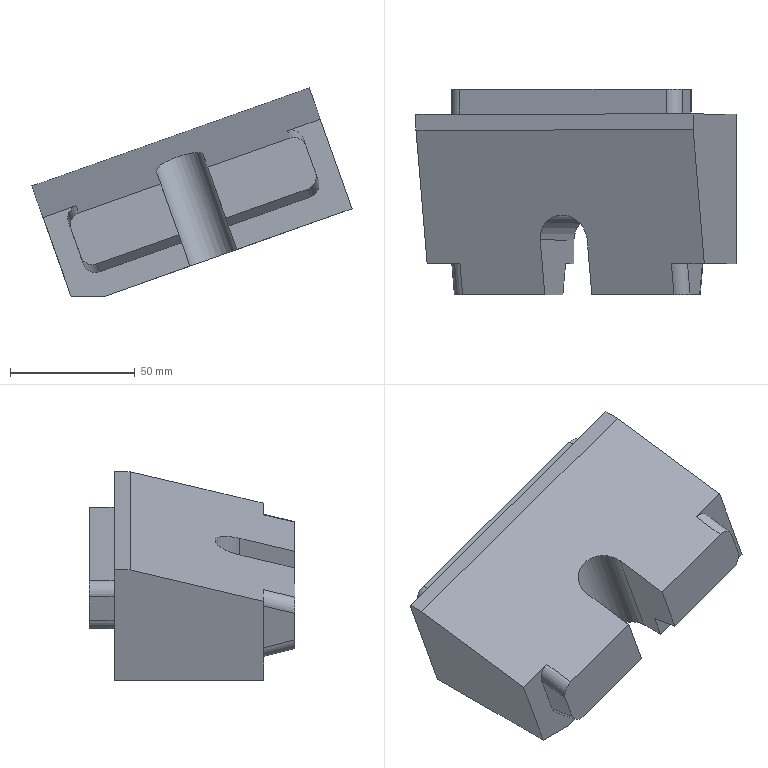Part | STEP file | WEDGE-1_id570_x_t | 1 solid | 31 faces | box 128.423 x 82.5 x 83.604 mm | volume 350596 mm3 | plane 22 | cylinder 9 | commonest cylinder face diameters 10 x8 20 x1
STEP:
#1=CARTESIAN_POINT('',(99.636,10.5,-205.83));
#2=VERTEX_POINT('',#1);
#3=CARTESIAN_POINT('',(16.683,10.5,-235.205));
#4=VERTEX_POINT('',#3);
#5=CARTESIAN_POINT('',(114.718,10.5,-200.489));
#6=DIRECTION('',(-0.9426,0.,-0.3338));
#7=VECTOR('',#6,1.);
#8=LINE('',#5,#7);
#9=EDGE_CURVE('',#2,#4,#8,.T.);
#10=ORIENTED_EDGE('',*,*,#9,.F.);
#11=CARTESIAN_POINT('',(106.018,10.5,-208.874));
#12=VERTEX_POINT('',#11);
#13=CARTESIAN_POINT('',(101.305,10.5,-210.543));
#14=DIRECTION('',(0.,-1.,0.));
#15=DIRECTION('',(0.,0.,1.));
#16=AXIS2_PLACEMENT_3D('',#13,#14,#15);
#17=CIRCLE('',#16,5.);
#18=EDGE_CURVE('',#12,#2,#17,.T.);
#19=ORIENTED_EDGE('',*,*,#18,.F.);
#20=CARTESIAN_POINT('',(109.356,10.5,-218.3));
#21=VERTEX_POINT('',#20);
#22=CARTESIAN_POINT('',(104.349,10.5,-204.16));
#23=DIRECTION('',(0.3338,0.,-0.9426));
#24=VECTOR('',#23,1.);
#25=LINE('',#22,#24);
#26=EDGE_CURVE('',#12,#21,#25,.T.);
#27=ORIENTED_EDGE('',*,*,#26,.T.);
#28=CARTESIAN_POINT('',(106.312,10.5,-224.682));
#29=VERTEX_POINT('',#28);
#30=CARTESIAN_POINT('',(104.643,10.5,-219.969));
#31=DIRECTION('',(0.,-1.,0.));
#32=DIRECTION('',(0.,0.,-1.));
#33=AXIS2_PLACEMENT_3D('',#30,#31,#32);
#34=CIRCLE('',#33,5.);
#35=EDGE_CURVE('',#29,#21,#34,.T.);
#36=ORIENTED_EDGE('',*,*,#35,.F.);
#37=CARTESIAN_POINT('',(23.359,10.5,-254.057));
#38=VERTEX_POINT('',#37);
#39=CARTESIAN_POINT('',(121.394,10.5,-219.341));
#40=DIRECTION('',(0.9426,0.,0.3338));
#41=VECTOR('',#40,1.);
#42=LINE('',#39,#41);
#43=EDGE_CURVE('',#38,#29,#42,.T.);
#44=ORIENTED_EDGE('',*,*,#43,.F.);
#45=CARTESIAN_POINT('',(16.977,10.5,-251.013));
#46=VERTEX_POINT('',#45);
#47=CARTESIAN_POINT('',(21.69,10.5,-249.344));
#48=DIRECTION('',(0.,-1.,0.));
#49=DIRECTION('',(0.,0.,1.));
#50=AXIS2_PLACEMENT_3D('',#47,#48,#49);
#51=CIRCLE('',#50,5.);
#52=EDGE_CURVE('',#46,#38,#51,.T.);
#53=ORIENTED_EDGE('',*,*,#52,.F.);
#54=CARTESIAN_POINT('',(13.639,10.5,-241.587));
#55=VERTEX_POINT('',#54);
#56=CARTESIAN_POINT('',(18.646,10.5,-255.726));
#57=DIRECTION('',(-0.3338,0.,0.9426));
#58=VECTOR('',#57,1.);
#59=LINE('',#56,#58);
#60=EDGE_CURVE('',#46,#55,#59,.T.);
#61=ORIENTED_EDGE('',*,*,#60,.T.);
#62=CARTESIAN_POINT('',(18.352,10.5,-239.918));
#63=DIRECTION('',(0.,-1.,0.));
#64=DIRECTION('',(0.,0.,-1.));
#65=AXIS2_PLACEMENT_3D('',#62,#63,#64);
#66=CIRCLE('',#65,5.);
#67=EDGE_CURVE('',#4,#55,#66,.T.);
#68=ORIENTED_EDGE('',*,*,#67,.F.);
#69=EDGE_LOOP('',(#10,#19,#27,#36,#44,#53,#61,#68));
#70=FACE_OUTER_BOUND('',#69,.T.);
#71=CARTESIAN_POINT('',(114.718,10.5,-200.489));
#72=DIRECTION('',(0.,1.,0.));
#73=DIRECTION('',(0.,0.,1.));
#74=AXIS2_PLACEMENT_3D('',#71,#72,#73);
#75=PLANE('',#74);
#76=ADVANCED_FACE('',(#70),#75,.T.);
#77=CARTESIAN_POINT('',(106.018,0.5,-208.874));
#78=VERTEX_POINT('',#77);
#79=CARTESIAN_POINT('',(99.636,0.5,-205.83));
#80=VERTEX_POINT('',#79);
#81=CARTESIAN_POINT('',(101.305,0.5,-210.543));
#82=DIRECTION('',(0.,-1.,0.));
#83=DIRECTION('',(0.,0.,1.));
#84=AXIS2_PLACEMENT_3D('',#81,#82,#83);
#85=CIRCLE('',#84,5.);
#86=EDGE_CURVE('',#78,#80,#85,.T.);
#87=ORIENTED_EDGE('',*,*,#86,.F.);
#88=CARTESIAN_POINT('',(106.018,0.5,-208.874));
#89=DIRECTION('',(0.,1.,0.));
#90=VECTOR('',#89,1.);
#91=LINE('',#88,#90);
#92=EDGE_CURVE('',#78,#12,#91,.T.);
#93=ORIENTED_EDGE('',*,*,#92,.T.);
#94=ORIENTED_EDGE('',*,*,#18,.T.);
#95=CARTESIAN_POINT('',(99.636,0.5,-205.83));
#96=DIRECTION('',(0.,1.,0.));
#97=VECTOR('',#96,1.);
#98=LINE('',#95,#97);
#99=EDGE_CURVE('',#80,#2,#98,.T.);
#100=ORIENTED_EDGE('',*,*,#99,.F.);
#101=EDGE_LOOP('',(#87,#93,#94,#100));
#102=FACE_OUTER_BOUND('',#101,.T.);
#103=CARTESIAN_POINT('',(101.305,0.2133,-210.543));
#104=DIRECTION('',(0.,1.,0.));
#105=DIRECTION('',(0.,0.,1.));
#106=AXIS2_PLACEMENT_3D('',#103,#104,#105);
#107=CYLINDRICAL_SURFACE('',#106,5.);
#108=ADVANCED_FACE('',(#102),#107,.T.);
#109=CARTESIAN_POINT('',(16.683,0.5,-235.205));
#110=VERTEX_POINT('',#109);
#111=CARTESIAN_POINT('',(99.636,0.5,-205.83));
#112=DIRECTION('',(-0.9426,0.,-0.3338));
#113=VECTOR('',#112,1.);
#114=LINE('',#111,#113);
#115=EDGE_CURVE('',#80,#110,#114,.T.);
#116=ORIENTED_EDGE('',*,*,#115,.F.);
#117=ORIENTED_EDGE('',*,*,#99,.T.);
#118=ORIENTED_EDGE('',*,*,#9,.T.);
#119=CARTESIAN_POINT('',(16.683,10.738,-235.205));
#120=DIRECTION('',(0.,1.,0.));
#121=VECTOR('',#120,1.);
#122=LINE('',#119,#121);
#123=EDGE_CURVE('',#110,#4,#122,.T.);
#124=ORIENTED_EDGE('',*,*,#123,.F.);
#125=EDGE_LOOP('',(#116,#117,#118,#124));
#126=FACE_OUTER_BOUND('',#125,.T.);
#127=CARTESIAN_POINT('',(114.718,0.5,-200.489));
#128=DIRECTION('',(-0.3338,0.,0.9426));
#129=DIRECTION('',(0.9426,0.,0.3338));
#130=AXIS2_PLACEMENT_3D('',#127,#128,#129);
#131=PLANE('',#130);
#132=ADVANCED_FACE('',(#126),#131,.T.);
#133=ORIENTED_EDGE('',*,*,#67,.T.);
#134=CARTESIAN_POINT('',(13.639,0.5,-241.587));
#135=VERTEX_POINT('',#134);
#136=CARTESIAN_POINT('',(13.639,0.5,-241.587));
#137=DIRECTION('',(0.,-1.,0.));
#138=VECTOR('',#137,1.);
#139=LINE('',#136,#138);
#140=EDGE_CURVE('',#55,#135,#139,.T.);
#141=ORIENTED_EDGE('',*,*,#140,.T.);
#142=CARTESIAN_POINT('',(18.352,0.5,-239.918));
#143=DIRECTION('',(0.,-1.,0.));
#144=DIRECTION('',(0.,0.,-1.));
#145=AXIS2_PLACEMENT_3D('',#142,#143,#144);
#146=CIRCLE('',#145,5.);
#147=EDGE_CURVE('',#110,#135,#146,.T.);
#148=ORIENTED_EDGE('',*,*,#147,.F.);
#149=ORIENTED_EDGE('',*,*,#123,.T.);
#150=EDGE_LOOP('',(#133,#141,#148,#149));
#151=FACE_OUTER_BOUND('',#150,.T.);
#152=CARTESIAN_POINT('',(18.352,10.738,-239.918));
#153=DIRECTION('',(0.,-1.,0.));
#154=DIRECTION('',(0.,0.,-1.));
#155=AXIS2_PLACEMENT_3D('',#152,#153,#154);
#156=CYLINDRICAL_SURFACE('',#155,5.);
#157=ADVANCED_FACE('',(#151),#156,.T.);
#158=CARTESIAN_POINT('',(16.977,0.5,-251.013));
#159=VERTEX_POINT('',#158);
#160=CARTESIAN_POINT('',(16.977,0.237,-251.013));
#161=DIRECTION('',(0.,1.,0.));
#162=VECTOR('',#161,1.);
#163=LINE('',#160,#162);
#164=EDGE_CURVE('',#159,#46,#163,.T.);
#165=ORIENTED_EDGE('',*,*,#164,.F.);
#166=CARTESIAN_POINT('',(13.639,0.5,-241.587));
#167=DIRECTION('',(0.3338,0.,-0.9426));
#168=VECTOR('',#167,1.);
#169=LINE('',#166,#168);
#170=EDGE_CURVE('',#135,#159,#169,.T.);
#171=ORIENTED_EDGE('',*,*,#170,.F.);
#172=ORIENTED_EDGE('',*,*,#140,.F.);
#173=ORIENTED_EDGE('',*,*,#60,.F.);
#174=EDGE_LOOP('',(#165,#171,#172,#173));
#175=FACE_OUTER_BOUND('',#174,.T.);
#176=CARTESIAN_POINT('',(18.646,0.5,-255.726));
#177=DIRECTION('',(0.9426,0.,0.3338));
#178=DIRECTION('',(0.3338,0.,-0.9426));
#179=AXIS2_PLACEMENT_3D('',#176,#177,#178);
#180=PLANE('',#179);
#181=ADVANCED_FACE('',(#175),#180,.F.);
#182=CARTESIAN_POINT('',(23.359,0.5,-254.057));
#183=VERTEX_POINT('',#182);
#184=CARTESIAN_POINT('',(21.69,0.5,-249.344));
#185=DIRECTION('',(0.,-1.,0.));
#186=DIRECTION('',(0.,0.,1.));
#187=AXIS2_PLACEMENT_3D('',#184,#185,#186);
#188=CIRCLE('',#187,5.);
#189=EDGE_CURVE('',#159,#183,#188,.T.);
#190=ORIENTED_EDGE('',*,*,#189,.F.);
#191=ORIENTED_EDGE('',*,*,#164,.T.);
#192=ORIENTED_EDGE('',*,*,#52,.T.);
#193=CARTESIAN_POINT('',(23.359,10.5,-254.057));
#194=DIRECTION('',(0.,1.,0.));
#195=VECTOR('',#194,1.);
#196=LINE('',#193,#195);
#197=EDGE_CURVE('',#183,#38,#196,.T.);
#198=ORIENTED_EDGE('',*,*,#197,.F.);
#199=EDGE_LOOP('',(#190,#191,#192,#198));
#200=FACE_OUTER_BOUND('',#199,.T.);
#201=CARTESIAN_POINT('',(21.69,0.237,-249.344));
#202=DIRECTION('',(0.,1.,0.));
#203=DIRECTION('',(0.,0.,1.));
#204=AXIS2_PLACEMENT_3D('',#201,#202,#203);
#205=CYLINDRICAL_SURFACE('',#204,5.);
#206=ADVANCED_FACE('',(#200),#205,.T.);
#207=ORIENTED_EDGE('',*,*,#43,.T.);
#208=CARTESIAN_POINT('',(106.312,0.5,-224.682));
#209=VERTEX_POINT('',#208);
#210=CARTESIAN_POINT('',(106.312,10.738,-224.682));
#211=DIRECTION('',(0.,1.,0.));
#212=VECTOR('',#211,1.);
#213=LINE('',#210,#212);
#214=EDGE_CURVE('',#209,#29,#213,.T.);
#215=ORIENTED_EDGE('',*,*,#214,.F.);
#216=CARTESIAN_POINT('',(23.359,0.5,-254.057));
#217=DIRECTION('',(0.9426,0.,0.3338));
#218=VECTOR('',#217,1.);
#219=LINE('',#216,#218);
#220=EDGE_CURVE('',#183,#209,#219,.T.);
#221=ORIENTED_EDGE('',*,*,#220,.F.);
#222=ORIENTED_EDGE('',*,*,#197,.T.);
#223=EDGE_LOOP('',(#207,#215,#221,#222));
#224=FACE_OUTER_BOUND('',#223,.T.);
#225=CARTESIAN_POINT('',(121.394,10.5,-219.341));
#226=DIRECTION('',(0.3338,0.,-0.9426));
#227=DIRECTION('',(-0.9426,0.,-0.3338));
#228=AXIS2_PLACEMENT_3D('',#225,#226,#227);
#229=PLANE('',#228);
#230=ADVANCED_FACE('',(#224),#229,.T.);
#231=ORIENTED_EDGE('',*,*,#35,.T.);
#232=CARTESIAN_POINT('',(109.356,0.5,-218.3));
#233=VERTEX_POINT('',#232);
#234=CARTESIAN_POINT('',(109.356,0.5,-218.3));
#235=DIRECTION('',(0.,-1.,0.));
#236=VECTOR('',#235,1.);
#237=LINE('',#234,#236);
#238=EDGE_CURVE('',#21,#233,#237,.T.);
#239=ORIENTED_EDGE('',*,*,#238,.T.);
#240=CARTESIAN_POINT('',(104.643,0.5,-219.969));
#241=DIRECTION('',(0.,-1.,0.));
#242=DIRECTION('',(0.,0.,-1.));
#243=AXIS2_PLACEMENT_3D('',#240,#241,#242);
#244=CIRCLE('',#243,5.);
#245=EDGE_CURVE('',#209,#233,#244,.T.);
#246=ORIENTED_EDGE('',*,*,#245,.F.);
#247=ORIENTED_EDGE('',*,*,#214,.T.);
#248=EDGE_LOOP('',(#231,#239,#246,#247));
#249=FACE_OUTER_BOUND('',#248,.T.);
#250=CARTESIAN_POINT('',(104.643,10.738,-219.969));
#251=DIRECTION('',(0.,-1.,0.));
#252=DIRECTION('',(0.,0.,-1.));
#253=AXIS2_PLACEMENT_3D('',#250,#251,#252);
#254=CYLINDRICAL_SURFACE('',#253,5.);
#255=ADVANCED_FACE('',(#249),#254,.T.);
#256=ORIENTED_EDGE('',*,*,#238,.F.);
#257=ORIENTED_EDGE('',*,*,#26,.F.);
#258=ORIENTED_EDGE('',*,*,#92,.F.);
#259=CARTESIAN_POINT('',(109.356,0.5,-218.3));
#260=DIRECTION('',(-0.3338,0.,0.9426));
#261=VECTOR('',#260,1.);
#262=LINE('',#259,#261);
#263=EDGE_CURVE('',#233,#78,#262,.T.);
#264=ORIENTED_EDGE('',*,*,#263,.F.);
#265=EDGE_LOOP('',(#256,#257,#258,#264));
#266=FACE_OUTER_BOUND('',#265,.T.);
#267=CARTESIAN_POINT('',(104.349,0.5,-204.16));
#268=DIRECTION('',(-0.9426,0.,-0.3338));
#269=DIRECTION('',(-0.3338,0.,0.9426));
#270=AXIS2_PLACEMENT_3D('',#267,#268,#269);
#271=PLANE('',#270);
#272=ADVANCED_FACE('',(#266),#271,.F.);
#273=CARTESIAN_POINT('',(109.174,-72.,-214.791));
#274=VERTEX_POINT('',#273);
#275=CARTESIAN_POINT('',(108.134,-59.5,-211.853));
#276=VERTEX_POINT('',#275);
#277=CARTESIAN_POINT('',(109.215,-72.495,-214.907));
#278=DIRECTION('',(-0.08076,0.9703,0.228));
#279=VECTOR('',#278,1.);
#280=LINE('',#277,#279);
#281=EDGE_CURVE('',#274,#276,#280,.T.);
#282=ORIENTED_EDGE('',*,*,#281,.F.);
#283=CARTESIAN_POINT('',(112.96,-72.,-225.483));
#284=VERTEX_POINT('',#283);
#285=CARTESIAN_POINT('',(112.96,-72.,-225.483));
#286=DIRECTION('',(-0.3338,0.,0.9426));
#287=VECTOR('',#286,1.);
#288=LINE('',#285,#287);
#289=EDGE_CURVE('',#284,#274,#288,.T.);
#290=ORIENTED_EDGE('',*,*,#289,.F.);
#291=CARTESIAN_POINT('',(114.078,-59.5,-228.64));
#292=VERTEX_POINT('',#291);
#293=CARTESIAN_POINT('',(114.222,-57.895,-229.046));
#294=DIRECTION('',(-0.0864,-0.9659,0.244));
#295=VECTOR('',#294,1.);
#296=LINE('',#293,#295);
#297=EDGE_CURVE('',#292,#284,#296,.T.);
#298=ORIENTED_EDGE('',*,*,#297,.F.);
#299=CARTESIAN_POINT('',(108.134,-59.5,-211.853));
#300=DIRECTION('',(0.3338,0.,-0.9426));
#301=VECTOR('',#300,1.);
#302=LINE('',#299,#301);
#303=EDGE_CURVE('',#276,#292,#302,.T.);
#304=ORIENTED_EDGE('',*,*,#303,.F.);
#305=EDGE_LOOP('',(#282,#290,#298,#304));
#306=FACE_OUTER_BOUND('',#305,.T.);
#307=CARTESIAN_POINT('',(104.791,-72.,-202.413));
#308=DIRECTION('',(-0.9426,0.,-0.3338));
#309=DIRECTION('',(-0.3338,0.,0.9426));
#310=AXIS2_PLACEMENT_3D('',#307,#308,#309);
#311=PLANE('',#310);
#312=ADVANCED_FACE('',(#306),#311,.F.);
#313=CARTESIAN_POINT('',(111.093,-59.5,-235.189));
#314=VERTEX_POINT('',#313);
#315=CARTESIAN_POINT('',(109.365,-59.5,-230.309));
#316=DIRECTION('',(0.,1.,0.));
#317=DIRECTION('',(-0.3338,0.,0.9426));
#318=AXIS2_PLACEMENT_3D('',#315,#316,#317);
#319=ELLIPSE('',#318,5.176,5.);
#320=EDGE_CURVE('',#292,#314,#319,.T.);
#321=ORIENTED_EDGE('',*,*,#320,.F.);
#322=ORIENTED_EDGE('',*,*,#297,.T.);
#323=CARTESIAN_POINT('',(109.975,-72.,-232.032));
#324=VERTEX_POINT('',#323);
#325=CARTESIAN_POINT('',(108.247,-72.,-227.152));
#326=DIRECTION('',(0.,-1.,0.));
#327=DIRECTION('',(-0.3338,0.,0.9426));
#328=AXIS2_PLACEMENT_3D('',#325,#326,#327);
#329=ELLIPSE('',#328,5.176,5.);
#330=EDGE_CURVE('',#324,#284,#329,.T.);
#331=ORIENTED_EDGE('',*,*,#330,.F.);
#332=CARTESIAN_POINT('',(111.093,-59.5,-235.189));
#333=DIRECTION('',(-0.0864,-0.9659,0.244));
#334=VECTOR('',#333,1.);
#335=LINE('',#332,#334);
#336=EDGE_CURVE('',#314,#324,#335,.T.);
#337=ORIENTED_EDGE('',*,*,#336,.F.);
#338=EDGE_LOOP('',(#321,#322,#331,#337));
#339=FACE_OUTER_BOUND('',#338,.T.);
#340=CARTESIAN_POINT('',(109.509,-57.895,-230.715));
#341=DIRECTION('',(-0.0864,-0.9659,0.244));
#342=DIRECTION('',(0.,-0.2449,-0.9696));
#343=AXIS2_PLACEMENT_3D('',#340,#341,#342);
#344=CYLINDRICAL_SURFACE('',#343,5.);
#345=ADVANCED_FACE('',(#339),#344,.T.);
#346=CARTESIAN_POINT('',(76.983,-72.,-243.715));
#347=VERTEX_POINT('',#346);
#348=CARTESIAN_POINT('',(76.983,-72.,-243.715));
#349=DIRECTION('',(0.9426,0.,0.3338));
#350=VECTOR('',#349,1.);
#351=LINE('',#348,#350);
#352=EDGE_CURVE('',#347,#324,#351,.T.);
#353=ORIENTED_EDGE('',*,*,#352,.F.);
#354=CARTESIAN_POINT('',(78.101,-59.5,-246.872));
#355=VERTEX_POINT('',#354);
#356=CARTESIAN_POINT('',(76.983,-72.,-243.715));
#357=DIRECTION('',(0.0864,0.9659,-0.244));
#358=VECTOR('',#357,1.);
#359=LINE('',#356,#358);
#360=EDGE_CURVE('',#347,#355,#359,.T.);
#361=ORIENTED_EDGE('',*,*,#360,.T.);
#362=CARTESIAN_POINT('',(111.093,-59.5,-235.189));
#363=DIRECTION('',(-0.9426,0.,-0.3338));
#364=VECTOR('',#363,1.);
#365=LINE('',#362,#364);
#366=EDGE_CURVE('',#314,#355,#365,.T.);
#367=ORIENTED_EDGE('',*,*,#366,.F.);
#368=ORIENTED_EDGE('',*,*,#336,.T.);
#369=EDGE_LOOP('',(#353,#361,#367,#368));
#370=FACE_OUTER_BOUND('',#369,.T.);
#371=CARTESIAN_POINT('',(125.233,-59.5,-230.182));
#372=DIRECTION('',(0.3224,-0.2588,-0.9105));
#373=DIRECTION('',(-0.9426,0.,-0.3338));
#374=AXIS2_PLACEMENT_3D('',#371,#372,#373);
#375=PLANE('',#374);
#376=ADVANCED_FACE('',(#370),#375,.T.);
#377=ORIENTED_EDGE('',*,*,#245,.T.);
#378=ORIENTED_EDGE('',*,*,#263,.T.);
#379=ORIENTED_EDGE('',*,*,#86,.T.);
#380=ORIENTED_EDGE('',*,*,#115,.T.);
#381=ORIENTED_EDGE('',*,*,#147,.T.);
#382=ORIENTED_EDGE('',*,*,#170,.T.);
#383=ORIENTED_EDGE('',*,*,#189,.T.);
#384=ORIENTED_EDGE('',*,*,#220,.T.);
#385=EDGE_LOOP('',(#377,#378,#379,#380,#381,#382,#383,#384));
#386=FACE_BOUND('',#385,.T.);
#387=CARTESIAN_POINT('',(28.628,0.5,-275.));
#388=VERTEX_POINT('',#387);
#389=CARTESIAN_POINT('',(14.863,0.5,-275.));
#390=VERTEX_POINT('',#389);
#391=CARTESIAN_POINT('',(14.863,0.5,-275.));
#392=DIRECTION('',(-1.,0.,0.));
#393=VECTOR('',#392,1.);
#394=LINE('',#391,#393);
#395=EDGE_CURVE('',#388,#390,#394,.T.);
#396=ORIENTED_EDGE('',*,*,#395,.T.);
#397=CARTESIAN_POINT('',(-0.7945,0.5,-230.785));
#398=VERTEX_POINT('',#397);
#399=CARTESIAN_POINT('',(16.397,0.5,-279.331));
#400=DIRECTION('',(-0.3338,0.,0.9426));
#401=VECTOR('',#400,1.);
#402=LINE('',#399,#401);
#403=EDGE_CURVE('',#390,#398,#402,.T.);
#404=ORIENTED_EDGE('',*,*,#403,.T.);
#405=CARTESIAN_POINT('',(110.437,0.5,-191.396));
#406=VERTEX_POINT('',#405);
#407=CARTESIAN_POINT('',(111.38,0.5,-191.062));
#408=DIRECTION('',(-0.9426,0.,-0.3338));
#409=VECTOR('',#408,1.);
#410=LINE('',#407,#409);
#411=EDGE_CURVE('',#406,#398,#410,.T.);
#412=ORIENTED_EDGE('',*,*,#411,.F.);
#413=CARTESIAN_POINT('',(127.628,0.5,-239.942));
#414=VERTEX_POINT('',#413);
#415=CARTESIAN_POINT('',(127.628,0.5,-239.942));
#416=DIRECTION('',(0.3338,0.,-0.9426));
#417=VECTOR('',#416,1.);
#418=LINE('',#415,#417);
#419=EDGE_CURVE('',#406,#414,#418,.T.);
#420=ORIENTED_EDGE('',*,*,#419,.T.);
#421=CARTESIAN_POINT('',(128.571,0.5,-239.608));
#422=DIRECTION('',(0.9426,0.,0.3338));
#423=VECTOR('',#422,1.);
#424=LINE('',#421,#423);
#425=EDGE_CURVE('',#388,#414,#424,.T.);
#426=ORIENTED_EDGE('',*,*,#425,.F.);
#427=EDGE_LOOP('',(#396,#404,#412,#420,#426));
#428=FACE_BOUND('',#427,.T.);
#429=CARTESIAN_POINT('',(111.38,0.5,-191.062));
#430=DIRECTION('',(0.,1.,0.));
#431=DIRECTION('',(0.,0.,1.));
#432=AXIS2_PLACEMENT_3D('',#429,#430,#431);
#433=PLANE('',#432);
#434=ADVANCED_FACE('',(#386,#428),#433,.T.);
#435=ORIENTED_EDGE('',*,*,#395,.F.);
#436=CARTESIAN_POINT('',(28.628,-59.5,-275.));
#437=VERTEX_POINT('',#436);
#438=CARTESIAN_POINT('',(28.628,0.5,-275.));
#439=DIRECTION('',(0.,1.,0.));
#440=VECTOR('',#439,1.);
#441=LINE('',#438,#440);
#442=EDGE_CURVE('',#437,#388,#441,.T.);
#443=ORIENTED_EDGE('',*,*,#442,.F.);
#444=CARTESIAN_POINT('',(14.863,-59.5,-275.));
#445=VERTEX_POINT('',#444);
#446=CARTESIAN_POINT('',(128.571,-59.5,-275.));
#447=DIRECTION('',(1.,0.,0.));
#448=VECTOR('',#447,1.);
#449=LINE('',#446,#448);
#450=EDGE_CURVE('',#445,#437,#449,.T.);
#451=ORIENTED_EDGE('',*,*,#450,.F.);
#452=CARTESIAN_POINT('',(14.863,10.5,-275.));
#453=DIRECTION('',(0.,1.,0.));
#454=VECTOR('',#453,1.);
#455=LINE('',#452,#454);
#456=EDGE_CURVE('',#445,#390,#455,.T.);
#457=ORIENTED_EDGE('',*,*,#456,.T.);
#458=EDGE_LOOP('',(#435,#443,#451,#457));
#459=FACE_OUTER_BOUND('',#458,.T.);
#460=CARTESIAN_POINT('',(14.863,0.5,-275.));
#461=DIRECTION('',(0.,0.,1.));
#462=DIRECTION('',(1.,0.,0.));
#463=AXIS2_PLACEMENT_3D('',#460,#461,#462);
#464=PLANE('',#463);
#465=ADVANCED_FACE('',(#459),#464,.F.);
#466=CARTESIAN_POINT('',(18.696,-72.,-258.864));
#467=VERTEX_POINT('',#466);
#468=CARTESIAN_POINT('',(19.814,-59.5,-262.021));
#469=VERTEX_POINT('',#468);
#470=CARTESIAN_POINT('',(18.657,-72.437,-258.753));
#471=DIRECTION('',(0.0864,0.9659,-0.244));
#472=VECTOR('',#471,1.);
#473=LINE('',#470,#472);
#474=EDGE_CURVE('',#467,#469,#473,.T.);
#475=ORIENTED_EDGE('',*,*,#474,.F.);
#476=CARTESIAN_POINT('',(14.91,-72.,-248.172));
#477=VERTEX_POINT('',#476);
#478=CARTESIAN_POINT('',(14.91,-72.,-248.172));
#479=DIRECTION('',(0.3338,0.,-0.9426));
#480=VECTOR('',#479,1.);
#481=LINE('',#478,#480);
#482=EDGE_CURVE('',#477,#467,#481,.T.);
#483=ORIENTED_EDGE('',*,*,#482,.F.);
#484=CARTESIAN_POINT('',(13.87,-59.5,-245.234));
#485=VERTEX_POINT('',#484);
#486=CARTESIAN_POINT('',(9.275,-4.289,-232.258));
#487=DIRECTION('',(0.08076,-0.9703,-0.228));
#488=VECTOR('',#487,1.);
#489=LINE('',#486,#488);
#490=EDGE_CURVE('',#485,#477,#489,.T.);
#491=ORIENTED_EDGE('',*,*,#490,.F.);
#492=CARTESIAN_POINT('',(19.814,-59.5,-262.021));
#493=DIRECTION('',(-0.3338,0.,0.9426));
#494=VECTOR('',#493,1.);
#495=LINE('',#492,#494);
#496=EDGE_CURVE('',#469,#485,#495,.T.);
#497=ORIENTED_EDGE('',*,*,#496,.F.);
#498=EDGE_LOOP('',(#475,#483,#491,#497));
#499=FACE_OUTER_BOUND('',#498,.T.);
#500=CARTESIAN_POINT('',(24.88,-72.,-276.327));
#501=DIRECTION('',(0.9426,0.,0.3338));
#502=DIRECTION('',(0.3338,0.,-0.9426));
#503=AXIS2_PLACEMENT_3D('',#500,#501,#502);
#504=PLANE('',#503);
#505=ADVANCED_FACE('',(#499),#504,.F.);
#506=CARTESIAN_POINT('',(25.137,-72.,-262.074));
#507=VERTEX_POINT('',#506);
#508=CARTESIAN_POINT('',(23.409,-72.,-257.195));
#509=DIRECTION('',(0.,-1.,0.));
#510=DIRECTION('',(0.3338,0.,-0.9426));
#511=AXIS2_PLACEMENT_3D('',#508,#509,#510);
#512=ELLIPSE('',#511,5.176,5.);
#513=EDGE_CURVE('',#467,#507,#512,.T.);
#514=ORIENTED_EDGE('',*,*,#513,.F.);
#515=ORIENTED_EDGE('',*,*,#474,.T.);
#516=CARTESIAN_POINT('',(26.255,-59.5,-265.232));
#517=VERTEX_POINT('',#516);
#518=CARTESIAN_POINT('',(24.528,-59.5,-260.352));
#519=DIRECTION('',(0.,1.,0.));
#520=DIRECTION('',(0.3338,0.,-0.9426));
#521=AXIS2_PLACEMENT_3D('',#518,#519,#520);
#522=ELLIPSE('',#521,5.176,5.);
#523=EDGE_CURVE('',#517,#469,#522,.T.);
#524=ORIENTED_EDGE('',*,*,#523,.F.);
#525=CARTESIAN_POINT('',(26.255,-59.5,-265.232));
#526=DIRECTION('',(0.0864,0.9659,-0.244));
#527=VECTOR('',#526,1.);
#528=LINE('',#525,#527);
#529=EDGE_CURVE('',#507,#517,#528,.T.);
#530=ORIENTED_EDGE('',*,*,#529,.F.);
#531=EDGE_LOOP('',(#514,#515,#524,#530));
#532=FACE_OUTER_BOUND('',#531,.T.);
#533=CARTESIAN_POINT('',(23.37,-72.437,-257.084));
#534=DIRECTION('',(0.0864,0.9659,-0.244));
#535=DIRECTION('',(0.,0.2449,0.9696));
#536=AXIS2_PLACEMENT_3D('',#533,#534,#535);
#537=CYLINDRICAL_SURFACE('',#536,5.);
#538=ADVANCED_FACE('',(#532),#537,.T.);
#539=CARTESIAN_POINT('',(59.248,-59.5,-253.548));
#540=VERTEX_POINT('',#539);
#541=CARTESIAN_POINT('',(59.248,-59.5,-253.548));
#542=DIRECTION('',(-0.9426,0.,-0.3338));
#543=VECTOR('',#542,1.);
#544=LINE('',#541,#543);
#545=EDGE_CURVE('',#540,#517,#544,.T.);
#546=ORIENTED_EDGE('',*,*,#545,.F.);
#547=CARTESIAN_POINT('',(58.13,-72.,-250.391));
#548=VERTEX_POINT('',#547);
#549=CARTESIAN_POINT('',(59.248,-59.5,-253.548));
#550=DIRECTION('',(-0.0864,-0.9659,0.244));
#551=VECTOR('',#550,1.);
#552=LINE('',#549,#551);
#553=EDGE_CURVE('',#540,#548,#552,.T.);
#554=ORIENTED_EDGE('',*,*,#553,.T.);
#555=CARTESIAN_POINT('',(25.137,-72.,-262.074));
#556=DIRECTION('',(0.9426,0.,0.3338));
#557=VECTOR('',#556,1.);
#558=LINE('',#555,#557);
#559=EDGE_CURVE('',#507,#548,#558,.T.);
#560=ORIENTED_EDGE('',*,*,#559,.F.);
#561=ORIENTED_EDGE('',*,*,#529,.T.);
#562=EDGE_LOOP('',(#546,#554,#560,#561));
#563=FACE_OUTER_BOUND('',#562,.T.);
#564=CARTESIAN_POINT('',(125.233,-59.5,-230.182));
#565=DIRECTION('',(0.3224,-0.2588,-0.9105));
#566=DIRECTION('',(-0.9426,0.,-0.3338));
#567=AXIS2_PLACEMENT_3D('',#564,#565,#566);
#568=PLANE('',#567);
#569=ADVANCED_FACE('',(#563),#568,.T.);
#570=CARTESIAN_POINT('',(81.439,-59.5,-256.299));
#571=VERTEX_POINT('',#570);
#572=CARTESIAN_POINT('',(81.439,-50.,-256.299));
#573=VERTEX_POINT('',#572);
#574=CARTESIAN_POINT('',(81.439,-76.822,-256.299));
#575=DIRECTION('',(0.,1.,0.));
#576=VECTOR('',#575,1.);
#577=LINE('',#574,#576);
#578=EDGE_CURVE('',#571,#573,#577,.T.);
#579=ORIENTED_EDGE('',*,*,#578,.T.);
#580=CARTESIAN_POINT('',(62.586,-50.,-262.975));
#581=VERTEX_POINT('',#580);
#582=CARTESIAN_POINT('',(72.012,-50.,-259.637));
#583=DIRECTION('',(-0.3338,0.,0.9426));
#584=DIRECTION('',(0.9426,0.,0.3338));
#585=AXIS2_PLACEMENT_3D('',#582,#583,#584);
#586=CIRCLE('',#585,10.);
#587=EDGE_CURVE('',#573,#581,#586,.T.);
#588=ORIENTED_EDGE('',*,*,#587,.T.);
#589=CARTESIAN_POINT('',(62.586,-59.5,-262.975));
#590=VERTEX_POINT('',#589);
#591=CARTESIAN_POINT('',(62.586,-50.,-262.975));
#592=DIRECTION('',(0.,-1.,0.));
#593=VECTOR('',#592,1.);
#594=LINE('',#591,#593);
#595=EDGE_CURVE('',#581,#590,#594,.T.);
#596=ORIENTED_EDGE('',*,*,#595,.T.);
#597=CARTESIAN_POINT('',(28.628,-59.5,-275.));
#598=DIRECTION('',(0.9426,0.,0.3338));
#599=VECTOR('',#598,1.);
#600=LINE('',#597,#599);
#601=EDGE_CURVE('',#437,#590,#600,.T.);
#602=ORIENTED_EDGE('',*,*,#601,.F.);
#603=ORIENTED_EDGE('',*,*,#442,.T.);
#604=ORIENTED_EDGE('',*,*,#425,.T.);
#605=CARTESIAN_POINT('',(127.628,-59.5,-239.942));
#606=VERTEX_POINT('',#605);
#607=CARTESIAN_POINT('',(127.628,-72.,-239.942));
#608=DIRECTION('',(0.,-1.,0.));
#609=VECTOR('',#608,1.);
#610=LINE('',#607,#609);
#611=EDGE_CURVE('',#414,#606,#610,.T.);
#612=ORIENTED_EDGE('',*,*,#611,.T.);
#613=CARTESIAN_POINT('',(81.439,-59.5,-256.299));
#614=DIRECTION('',(0.9426,0.,0.3338));
#615=VECTOR('',#614,1.);
#616=LINE('',#613,#615);
#617=EDGE_CURVE('',#571,#606,#616,.T.);
#618=ORIENTED_EDGE('',*,*,#617,.F.);
#619=EDGE_LOOP('',(#579,#588,#596,#602,#603,#604,#612,#618));
#620=FACE_OUTER_BOUND('',#619,.T.);
#621=CARTESIAN_POINT('',(128.571,0.5,-239.608));
#622=DIRECTION('',(0.3338,0.,-0.9426));
#623=DIRECTION('',(-0.9426,0.,-0.3338));
#624=AXIS2_PLACEMENT_3D('',#621,#622,#623);
#625=PLANE('',#624);
#626=ADVANCED_FACE('',(#620),#625,.T.);
#627=ORIENTED_EDGE('',*,*,#578,.F.);
#628=CARTESIAN_POINT('',(78.101,-59.5,-246.872));
#629=DIRECTION('',(0.3338,0.,-0.9426));
#630=VECTOR('',#629,1.);
#631=LINE('',#628,#630);
#632=EDGE_CURVE('',#355,#571,#631,.T.);
#633=ORIENTED_EDGE('',*,*,#632,.F.);
#634=ORIENTED_EDGE('',*,*,#360,.F.);
#635=CARTESIAN_POINT('',(69.748,-72.,-223.286));
#636=VERTEX_POINT('',#635);
#637=CARTESIAN_POINT('',(69.748,-72.,-223.286));
#638=DIRECTION('',(0.3338,0.,-0.9426));
#639=VECTOR('',#638,1.);
#640=LINE('',#637,#639);
#641=EDGE_CURVE('',#636,#347,#640,.T.);
#642=ORIENTED_EDGE('',*,*,#641,.F.);
#643=CARTESIAN_POINT('',(67.917,-50.,-218.115));
#644=VERTEX_POINT('',#643);
#645=CARTESIAN_POINT('',(69.748,-72.,-223.286));
#646=DIRECTION('',(0.08076,-0.9703,-0.228));
#647=VECTOR('',#646,1.);
#648=LINE('',#645,#647);
#649=EDGE_CURVE('',#644,#636,#648,.T.);
#650=ORIENTED_EDGE('',*,*,#649,.F.);
#651=CARTESIAN_POINT('',(64.248,-50.,-207.753));
#652=DIRECTION('',(0.3338,0.,-0.9426));
#653=VECTOR('',#652,1.);
#654=LINE('',#651,#653);
#655=EDGE_CURVE('',#644,#573,#654,.T.);
#656=ORIENTED_EDGE('',*,*,#655,.T.);
#657=EDGE_LOOP('',(#627,#633,#634,#642,#650,#656));
#658=FACE_OUTER_BOUND('',#657,.T.);
#659=CARTESIAN_POINT('',(64.248,-76.822,-207.753));
#660=DIRECTION('',(0.9426,0.,0.3338));
#661=DIRECTION('',(0.3338,0.,-0.9426));
#662=AXIS2_PLACEMENT_3D('',#659,#660,#661);
#663=PLANE('',#662);
#664=ADVANCED_FACE('',(#658),#663,.F.);
#665=CARTESIAN_POINT('',(102.741,-72.,-211.603));
#666=VERTEX_POINT('',#665);
#667=CARTESIAN_POINT('',(116.88,-72.,-206.596));
#668=DIRECTION('',(0.9426,0.,0.3338));
#669=VECTOR('',#668,1.);
#670=LINE('',#667,#669);
#671=EDGE_CURVE('',#636,#666,#670,.T.);
#672=ORIENTED_EDGE('',*,*,#671,.F.);
#673=ORIENTED_EDGE('',*,*,#641,.T.);
#674=ORIENTED_EDGE('',*,*,#352,.T.);
#675=ORIENTED_EDGE('',*,*,#330,.T.);
#676=ORIENTED_EDGE('',*,*,#289,.T.);
#677=CARTESIAN_POINT('',(104.461,-72.,-216.46));
#678=DIRECTION('',(0.,1.,0.));
#679=DIRECTION('',(-0.3338,0.,0.9426));
#680=AXIS2_PLACEMENT_3D('',#677,#678,#679);
#681=ELLIPSE('',#680,5.153,5.);
#682=EDGE_CURVE('',#666,#274,#681,.T.);
#683=ORIENTED_EDGE('',*,*,#682,.F.);
#684=EDGE_LOOP('',(#672,#673,#674,#675,#676,#683));
#685=FACE_OUTER_BOUND('',#684,.T.);
#686=CARTESIAN_POINT('',(124.115,-72.,-227.025));
#687=DIRECTION('',(0.,-1.,0.));
#688=DIRECTION('',(0.,0.,-1.));
#689=AXIS2_PLACEMENT_3D('',#686,#687,#688);
#690=PLANE('',#689);
#691=ADVANCED_FACE('',(#685),#690,.T.);
#692=ORIENTED_EDGE('',*,*,#682,.T.);
#693=ORIENTED_EDGE('',*,*,#281,.T.);
#694=CARTESIAN_POINT('',(101.7,-59.5,-208.665));
#695=VERTEX_POINT('',#694);
#696=CARTESIAN_POINT('',(103.421,-59.5,-213.522));
#697=DIRECTION('',(0.,1.,0.));
#698=DIRECTION('',(-0.3338,0.,0.9426));
#699=AXIS2_PLACEMENT_3D('',#696,#697,#698);
#700=ELLIPSE('',#699,5.153,5.);
#701=EDGE_CURVE('',#695,#276,#700,.T.);
#702=ORIENTED_EDGE('',*,*,#701,.F.);
#703=CARTESIAN_POINT('',(102.741,-72.,-211.603));
#704=DIRECTION('',(-0.08076,0.9703,0.228));
#705=VECTOR('',#704,1.);
#706=LINE('',#703,#705);
#707=EDGE_CURVE('',#666,#695,#706,.T.);
#708=ORIENTED_EDGE('',*,*,#707,.F.);
#709=EDGE_LOOP('',(#692,#693,#702,#708));
#710=FACE_OUTER_BOUND('',#709,.T.);
#711=CARTESIAN_POINT('',(104.502,-72.495,-216.577));
#712=DIRECTION('',(-0.08076,0.9703,0.228));
#713=DIRECTION('',(0.,-0.2288,0.9735));
#714=AXIS2_PLACEMENT_3D('',#711,#712,#713);
#715=CYLINDRICAL_SURFACE('',#714,5.);
#716=ADVANCED_FACE('',(#710),#715,.T.);
#717=ORIENTED_EDGE('',*,*,#366,.T.);
#718=ORIENTED_EDGE('',*,*,#632,.T.);
#719=ORIENTED_EDGE('',*,*,#617,.T.);
#720=CARTESIAN_POINT('',(114.897,-59.5,-203.991));
#721=VERTEX_POINT('',#720);
#722=CARTESIAN_POINT('',(127.628,-59.5,-239.942));
#723=DIRECTION('',(-0.3338,0.,0.9426));
#724=VECTOR('',#723,1.);
#725=LINE('',#722,#724);
#726=EDGE_CURVE('',#606,#721,#725,.T.);
#727=ORIENTED_EDGE('',*,*,#726,.T.);
#728=CARTESIAN_POINT('',(115.84,-59.5,-203.658));
#729=DIRECTION('',(0.9426,0.,0.3338));
#730=VECTOR('',#729,1.);
#731=LINE('',#728,#730);
#732=EDGE_CURVE('',#695,#721,#731,.T.);
#733=ORIENTED_EDGE('',*,*,#732,.F.);
#734=ORIENTED_EDGE('',*,*,#701,.T.);
#735=ORIENTED_EDGE('',*,*,#303,.T.);
#736=ORIENTED_EDGE('',*,*,#320,.T.);
#737=EDGE_LOOP('',(#717,#718,#719,#727,#733,#734,#735,#736));
#738=FACE_OUTER_BOUND('',#737,.T.);
#739=CARTESIAN_POINT('',(128.571,-59.5,-239.608));
#740=DIRECTION('',(0.,-1.,0.));
#741=DIRECTION('',(0.,0.,-1.));
#742=AXIS2_PLACEMENT_3D('',#739,#740,#741);
#743=PLANE('',#742);
#744=ADVANCED_FACE('',(#738),#743,.T.);
#745=CARTESIAN_POINT('',(110.437,-5.908,-191.396));
#746=VERTEX_POINT('',#745);
#747=CARTESIAN_POINT('',(115.938,-72.,-206.929));
#748=DIRECTION('',(-0.08076,0.9703,0.228));
#749=VECTOR('',#748,1.);
#750=LINE('',#747,#749);
#751=EDGE_CURVE('',#721,#746,#750,.T.);
#752=ORIENTED_EDGE('',*,*,#751,.F.);
#753=ORIENTED_EDGE('',*,*,#726,.F.);
#754=ORIENTED_EDGE('',*,*,#611,.F.);
#755=ORIENTED_EDGE('',*,*,#419,.F.);
#756=CARTESIAN_POINT('',(110.437,-5.908,-191.396));
#757=DIRECTION('',(0.,1.,0.));
#758=VECTOR('',#757,1.);
#759=LINE('',#756,#758);
#760=EDGE_CURVE('',#746,#406,#759,.T.);
#761=ORIENTED_EDGE('',*,*,#760,.F.);
#762=EDGE_LOOP('',(#752,#753,#754,#755,#761));
#763=FACE_OUTER_BOUND('',#762,.T.);
#764=CARTESIAN_POINT('',(127.628,-72.,-239.942));
#765=DIRECTION('',(-0.9426,0.,-0.3338));
#766=DIRECTION('',(-0.3338,0.,0.9426));
#767=AXIS2_PLACEMENT_3D('',#764,#765,#766);
#768=PLANE('',#767);
#769=ADVANCED_FACE('',(#763),#768,.F.);
#770=ORIENTED_EDGE('',*,*,#411,.T.);
#771=CARTESIAN_POINT('',(-0.7945,-5.908,-230.785));
#772=VERTEX_POINT('',#771);
#773=CARTESIAN_POINT('',(-0.7945,10.5,-230.785));
#774=DIRECTION('',(0.,-1.,0.));
#775=VECTOR('',#774,1.);
#776=LINE('',#773,#775);
#777=EDGE_CURVE('',#398,#772,#776,.T.);
#778=ORIENTED_EDGE('',*,*,#777,.T.);
#779=CARTESIAN_POINT('',(111.38,-5.908,-191.062));
#780=DIRECTION('',(-0.9426,0.,-0.3338));
#781=VECTOR('',#780,1.);
#782=LINE('',#779,#781);
#783=EDGE_CURVE('',#746,#772,#782,.T.);
#784=ORIENTED_EDGE('',*,*,#783,.F.);
#785=ORIENTED_EDGE('',*,*,#760,.T.);
#786=EDGE_LOOP('',(#770,#778,#784,#785));
#787=FACE_OUTER_BOUND('',#786,.T.);
#788=CARTESIAN_POINT('',(111.38,-5.908,-191.062));
#789=DIRECTION('',(-0.3338,0.,0.9426));
#790=DIRECTION('',(0.9426,0.,0.3338));
#791=AXIS2_PLACEMENT_3D('',#788,#789,#790);
#792=PLANE('',#791);
#793=ADVANCED_FACE('',(#787),#792,.T.);
#794=CARTESIAN_POINT('',(3.666,-59.5,-243.381));
#795=VERTEX_POINT('',#794);
#796=CARTESIAN_POINT('',(3.666,-59.5,-243.381));
#797=DIRECTION('',(0.3338,0.,-0.9426));
#798=VECTOR('',#797,1.);
#799=LINE('',#796,#798);
#800=EDGE_CURVE('',#795,#445,#799,.T.);
#801=ORIENTED_EDGE('',*,*,#800,.F.);
#802=CARTESIAN_POINT('',(4.706,-72.,-246.319));
#803=DIRECTION('',(0.08076,-0.9703,-0.228));
#804=VECTOR('',#803,1.);
#805=LINE('',#802,#804);
#806=EDGE_CURVE('',#772,#795,#805,.T.);
#807=ORIENTED_EDGE('',*,*,#806,.F.);
#808=ORIENTED_EDGE('',*,*,#777,.F.);
#809=ORIENTED_EDGE('',*,*,#403,.F.);
#810=ORIENTED_EDGE('',*,*,#456,.F.);
#811=EDGE_LOOP('',(#801,#807,#808,#809,#810));
#812=FACE_OUTER_BOUND('',#811,.T.);
#813=CARTESIAN_POINT('',(16.397,10.5,-279.331));
#814=DIRECTION('',(0.9426,0.,0.3338));
#815=DIRECTION('',(0.3338,0.,-0.9426));
#816=AXIS2_PLACEMENT_3D('',#813,#814,#815);
#817=PLANE('',#816);
#818=ADVANCED_FACE('',(#812),#817,.F.);
#819=ORIENTED_EDGE('',*,*,#601,.T.);
#820=CARTESIAN_POINT('',(45.395,-59.5,-214.429));
#821=DIRECTION('',(-0.3338,0.,0.9426));
#822=VECTOR('',#821,1.);
#823=LINE('',#820,#822);
#824=EDGE_CURVE('',#590,#540,#823,.T.);
#825=ORIENTED_EDGE('',*,*,#824,.T.);
#826=ORIENTED_EDGE('',*,*,#545,.T.);
#827=ORIENTED_EDGE('',*,*,#523,.T.);
#828=ORIENTED_EDGE('',*,*,#496,.T.);
#829=CARTESIAN_POINT('',(16.863,-59.5,-238.707));
#830=VERTEX_POINT('',#829);
#831=CARTESIAN_POINT('',(18.583,-59.5,-243.565));
#832=DIRECTION('',(0.,-1.,0.));
#833=DIRECTION('',(0.3338,0.,-0.9426));
#834=AXIS2_PLACEMENT_3D('',#831,#832,#833);
#835=ELLIPSE('',#834,5.153,5.);
#836=EDGE_CURVE('',#830,#485,#835,.T.);
#837=ORIENTED_EDGE('',*,*,#836,.F.);
#838=CARTESIAN_POINT('',(115.84,-59.5,-203.658));
#839=DIRECTION('',(0.9426,0.,0.3338));
#840=VECTOR('',#839,1.);
#841=LINE('',#838,#840);
#842=EDGE_CURVE('',#795,#830,#841,.T.);
#843=ORIENTED_EDGE('',*,*,#842,.F.);
#844=ORIENTED_EDGE('',*,*,#800,.T.);
#845=ORIENTED_EDGE('',*,*,#450,.T.);
#846=EDGE_LOOP('',(#819,#825,#826,#827,#828,#837,#843,#844,#845));
#847=FACE_OUTER_BOUND('',#846,.T.);
#848=CARTESIAN_POINT('',(128.571,-59.5,-239.608));
#849=DIRECTION('',(0.,-1.,0.));
#850=DIRECTION('',(0.,0.,-1.));
#851=AXIS2_PLACEMENT_3D('',#848,#849,#850);
#852=PLANE('',#851);
#853=ADVANCED_FACE('',(#847),#852,.T.);
#854=ORIENTED_EDGE('',*,*,#836,.T.);
#855=ORIENTED_EDGE('',*,*,#490,.T.);
#856=CARTESIAN_POINT('',(17.903,-72.,-241.645));
#857=VERTEX_POINT('',#856);
#858=CARTESIAN_POINT('',(19.623,-72.,-246.503));
#859=DIRECTION('',(0.,-1.,0.));
#860=DIRECTION('',(0.3338,0.,-0.9426));
#861=AXIS2_PLACEMENT_3D('',#858,#859,#860);
#862=ELLIPSE('',#861,5.153,5.);
#863=EDGE_CURVE('',#857,#477,#862,.T.);
#864=ORIENTED_EDGE('',*,*,#863,.F.);
#865=CARTESIAN_POINT('',(17.903,-72.,-241.645));
#866=DIRECTION('',(0.08076,-0.9703,-0.228));
#867=VECTOR('',#866,1.);
#868=LINE('',#865,#867);
#869=EDGE_CURVE('',#830,#857,#868,.T.);
#870=ORIENTED_EDGE('',*,*,#869,.F.);
#871=EDGE_LOOP('',(#854,#855,#864,#870));
#872=FACE_OUTER_BOUND('',#871,.T.);
#873=CARTESIAN_POINT('',(13.988,-4.289,-230.589));
#874=DIRECTION('',(0.08076,-0.9703,-0.228));
#875=DIRECTION('',(0.,0.2288,-0.9735));
#876=AXIS2_PLACEMENT_3D('',#873,#874,#875);
#877=CYLINDRICAL_SURFACE('',#876,5.);
#878=ADVANCED_FACE('',(#872),#877,.T.);
#879=ORIENTED_EDGE('',*,*,#559,.T.);
#880=CARTESIAN_POINT('',(50.896,-72.,-229.962));
#881=VERTEX_POINT('',#880);
#882=CARTESIAN_POINT('',(45.395,-72.,-214.429));
#883=DIRECTION('',(-0.3338,0.,0.9426));
#884=VECTOR('',#883,1.);
#885=LINE('',#882,#884);
#886=EDGE_CURVE('',#548,#881,#885,.T.);
#887=ORIENTED_EDGE('',*,*,#886,.T.);
#888=CARTESIAN_POINT('',(116.88,-72.,-206.596));
#889=DIRECTION('',(0.9426,0.,0.3338));
#890=VECTOR('',#889,1.);
#891=LINE('',#888,#890);
#892=EDGE_CURVE('',#857,#881,#891,.T.);
#893=ORIENTED_EDGE('',*,*,#892,.F.);
#894=ORIENTED_EDGE('',*,*,#863,.T.);
#895=ORIENTED_EDGE('',*,*,#482,.T.);
#896=ORIENTED_EDGE('',*,*,#513,.T.);
#897=EDGE_LOOP('',(#879,#887,#893,#894,#895,#896));
#898=FACE_OUTER_BOUND('',#897,.T.);
#899=CARTESIAN_POINT('',(124.115,-72.,-227.025));
#900=DIRECTION('',(0.,-1.,0.));
#901=DIRECTION('',(0.,0.,-1.));
#902=AXIS2_PLACEMENT_3D('',#899,#900,#901);
#903=PLANE('',#902);
#904=ADVANCED_FACE('',(#898),#903,.T.);
#905=ORIENTED_EDGE('',*,*,#553,.F.);
#906=ORIENTED_EDGE('',*,*,#824,.F.);
#907=ORIENTED_EDGE('',*,*,#595,.F.);
#908=CARTESIAN_POINT('',(49.065,-50.,-224.791));
#909=VERTEX_POINT('',#908);
#910=CARTESIAN_POINT('',(45.395,-50.,-214.429));
#911=DIRECTION('',(-0.3338,0.,0.9426));
#912=VECTOR('',#911,1.);
#913=LINE('',#910,#912);
#914=EDGE_CURVE('',#581,#909,#913,.T.);
#915=ORIENTED_EDGE('',*,*,#914,.T.);
#916=CARTESIAN_POINT('',(50.896,-72.,-229.962));
#917=DIRECTION('',(-0.08076,0.9703,0.228));
#918=VECTOR('',#917,1.);
#919=LINE('',#916,#918);
#920=EDGE_CURVE('',#881,#909,#919,.T.);
#921=ORIENTED_EDGE('',*,*,#920,.F.);
#922=ORIENTED_EDGE('',*,*,#886,.F.);
#923=EDGE_LOOP('',(#905,#906,#907,#915,#921,#922));
#924=FACE_OUTER_BOUND('',#923,.T.);
#925=CARTESIAN_POINT('',(45.395,-50.,-214.429));
#926=DIRECTION('',(-0.9426,0.,-0.3338));
#927=DIRECTION('',(-0.3338,0.,0.9426));
#928=AXIS2_PLACEMENT_3D('',#925,#926,#927);
#929=PLANE('',#928);
#930=ADVANCED_FACE('',(#924),#929,.F.);
#931=ORIENTED_EDGE('',*,*,#587,.F.);
#932=ORIENTED_EDGE('',*,*,#655,.F.);
#933=CARTESIAN_POINT('',(58.491,-50.,-221.453));
#934=DIRECTION('',(0.3239,0.2419,-0.9146));
#935=DIRECTION('',(-0.08076,0.9703,0.228));
#936=AXIS2_PLACEMENT_3D('',#933,#934,#935);
#937=ELLIPSE('',#936,10.306,10.);
#938=EDGE_CURVE('',#909,#644,#937,.T.);
#939=ORIENTED_EDGE('',*,*,#938,.F.);
#940=ORIENTED_EDGE('',*,*,#914,.F.);
#941=EDGE_LOOP('',(#931,#932,#939,#940));
#942=FACE_OUTER_BOUND('',#941,.T.);
#943=CARTESIAN_POINT('',(54.821,-50.,-211.091));
#944=DIRECTION('',(-0.3338,0.,0.9426));
#945=DIRECTION('',(0.9426,0.,0.3338));
#946=AXIS2_PLACEMENT_3D('',#943,#944,#945);
#947=CYLINDRICAL_SURFACE('',#946,10.);
#948=ADVANCED_FACE('',(#942),#947,.F.);
#949=ORIENTED_EDGE('',*,*,#920,.T.);
#950=ORIENTED_EDGE('',*,*,#938,.T.);
#951=ORIENTED_EDGE('',*,*,#649,.T.);
#952=ORIENTED_EDGE('',*,*,#671,.T.);
#953=ORIENTED_EDGE('',*,*,#707,.T.);
#954=ORIENTED_EDGE('',*,*,#732,.T.);
#955=ORIENTED_EDGE('',*,*,#751,.T.);
#956=ORIENTED_EDGE('',*,*,#783,.T.);
#957=ORIENTED_EDGE('',*,*,#806,.T.);
#958=ORIENTED_EDGE('',*,*,#842,.T.);
#959=ORIENTED_EDGE('',*,*,#869,.T.);
#960=ORIENTED_EDGE('',*,*,#892,.T.);
#961=EDGE_LOOP('',(#949,#950,#951,#952,#953,#954,#955,#956,#957,#958,#959,#960));
#962=FACE_OUTER_BOUND('',#961,.T.);
#963=CARTESIAN_POINT('',(116.88,-72.,-206.596));
#964=DIRECTION('',(-0.3239,-0.2419,0.9146));
#965=DIRECTION('',(0.9426,0.,0.3338));
#966=AXIS2_PLACEMENT_3D('',#963,#964,#965);
#967=PLANE('',#966);
#968=ADVANCED_FACE('',(#962),#967,.T.);
#969=CLOSED_SHELL('',(#76,#108,#132,#157,#181,#206,#230,#255,#272,#312,#345,#376,#434,#465,#505,#538,#569,#626,#664,#691,#716,#744,#769,#793,#818,#853,#878,#904,#930,#948,#968));
#970=MANIFOLD_SOLID_BREP('',#969);
#971=(LENGTH_UNIT()NAMED_UNIT(*)SI_UNIT(.MILLI.,.METRE.));
#972=UNCERTAINTY_MEASURE_WITH_UNIT(LENGTH_MEASURE(0.00004123),#971,'','');
#973=(NAMED_UNIT(*)PLANE_ANGLE_UNIT()SI_UNIT($,.RADIAN.));
#974=PLANE_ANGLE_MEASURE_WITH_UNIT(PLANE_ANGLE_MEASURE(0.01745),#973);
#975=DIMENSIONAL_EXPONENTS(0.,0.,0.,0.,0.,0.,0.);
#976=(CONVERSION_BASED_UNIT('DEGREE',#974)NAMED_UNIT(#975)PLANE_ANGLE_UNIT());
#977=(NAMED_UNIT(*)SI_UNIT($,.STERADIAN.)SOLID_ANGLE_UNIT());
#978=(GEOMETRIC_REPRESENTATION_CONTEXT(3)GLOBAL_UNCERTAINTY_ASSIGNED_CONTEXT((#972))GLOBAL_UNIT_ASSIGNED_CONTEXT((#971,#976,#977))REPRESENTATION_CONTEXT('',''));
#979=ADVANCED_BREP_SHAPE_REPRESENTATION('',(#970),#978);